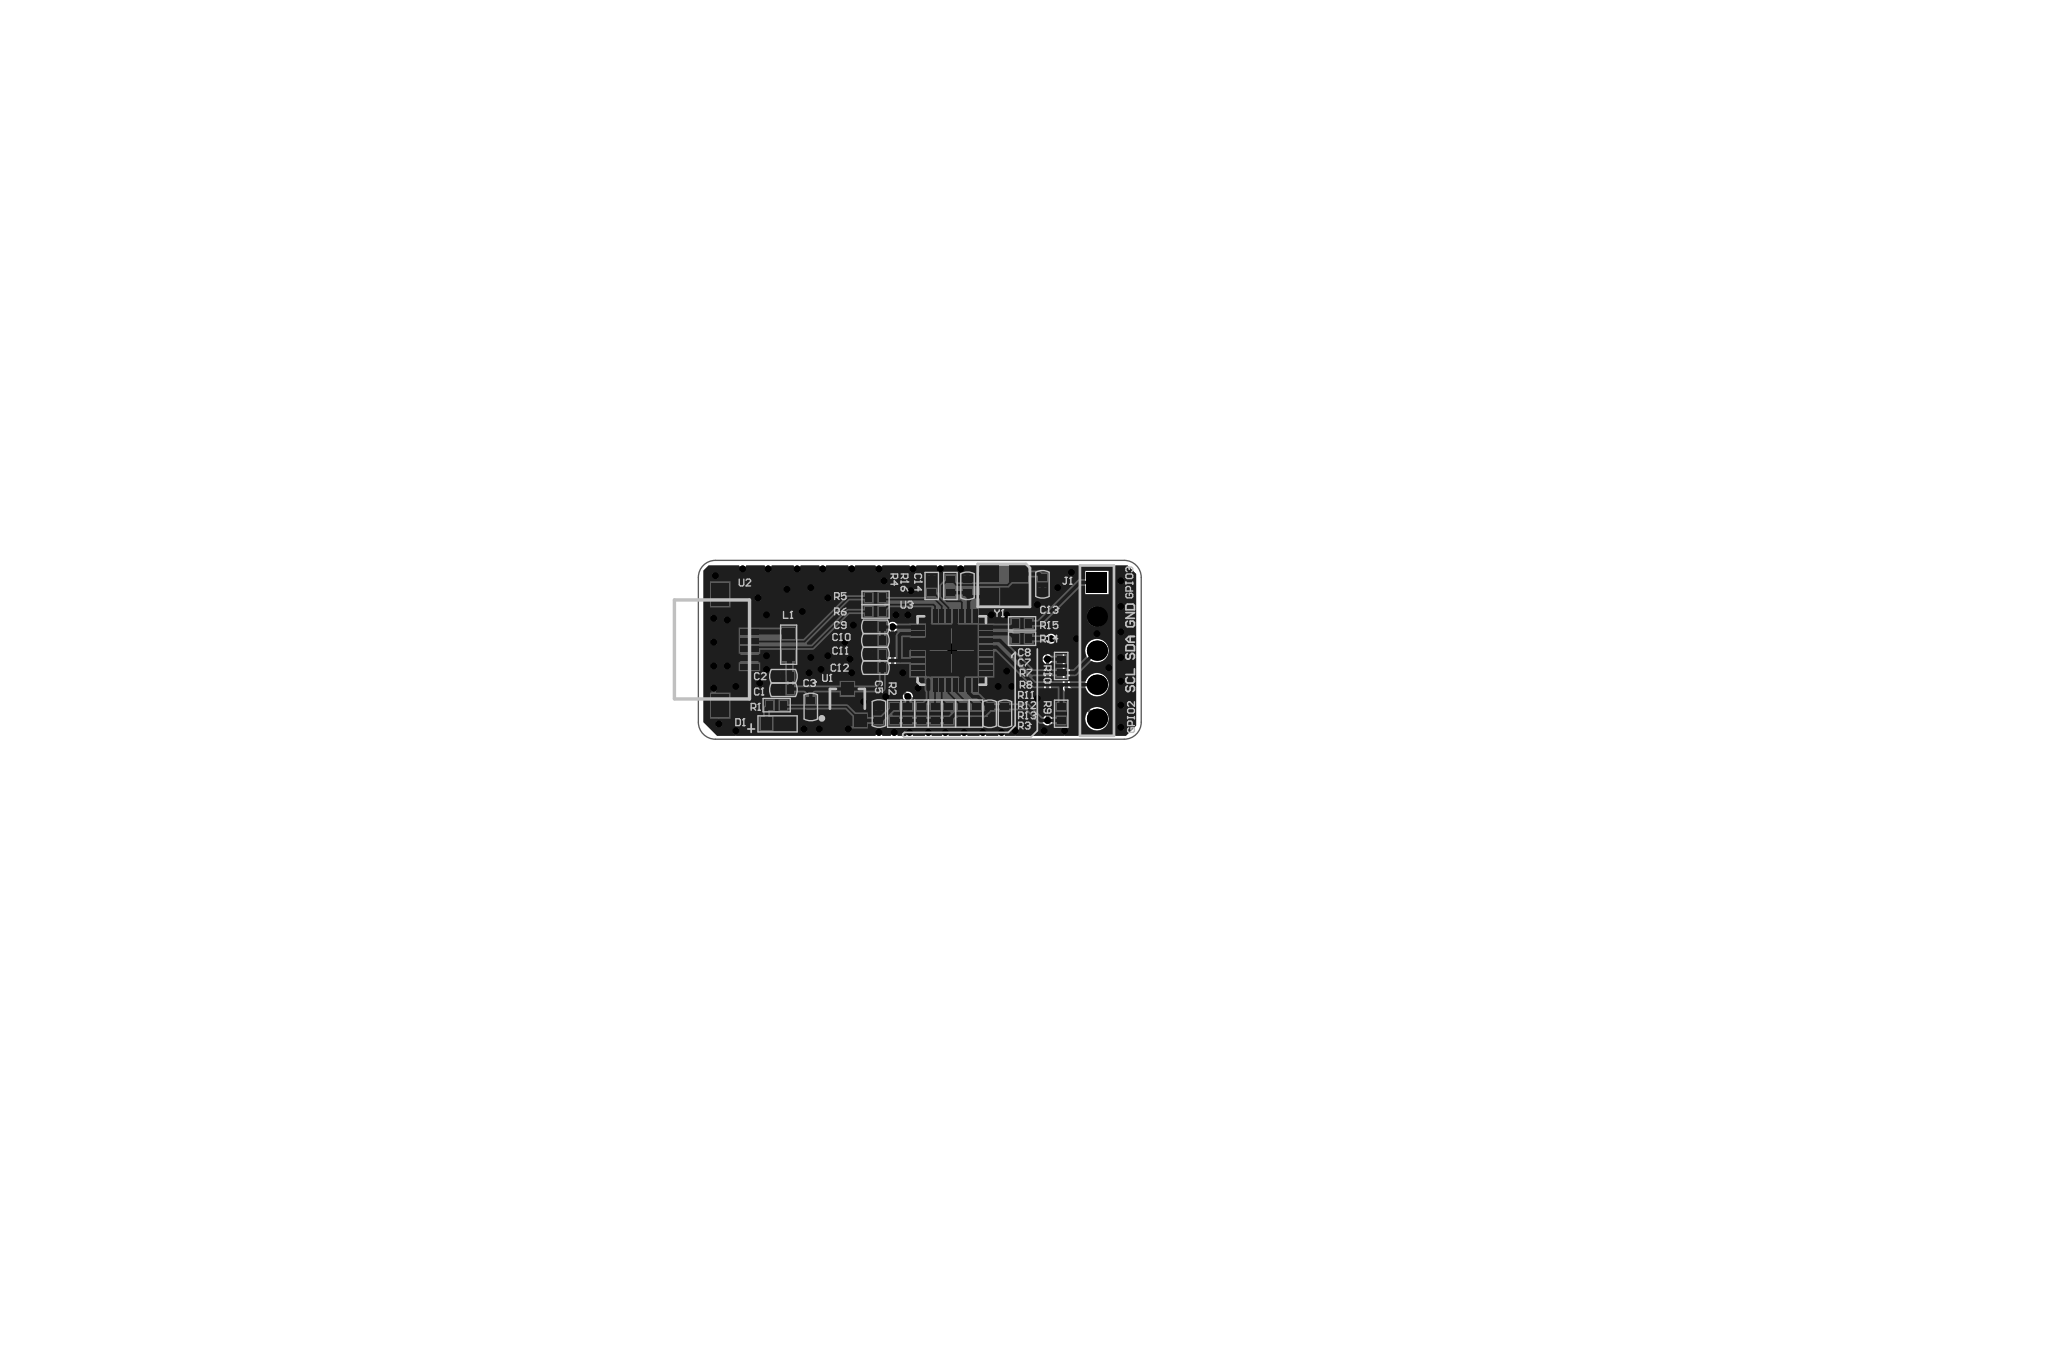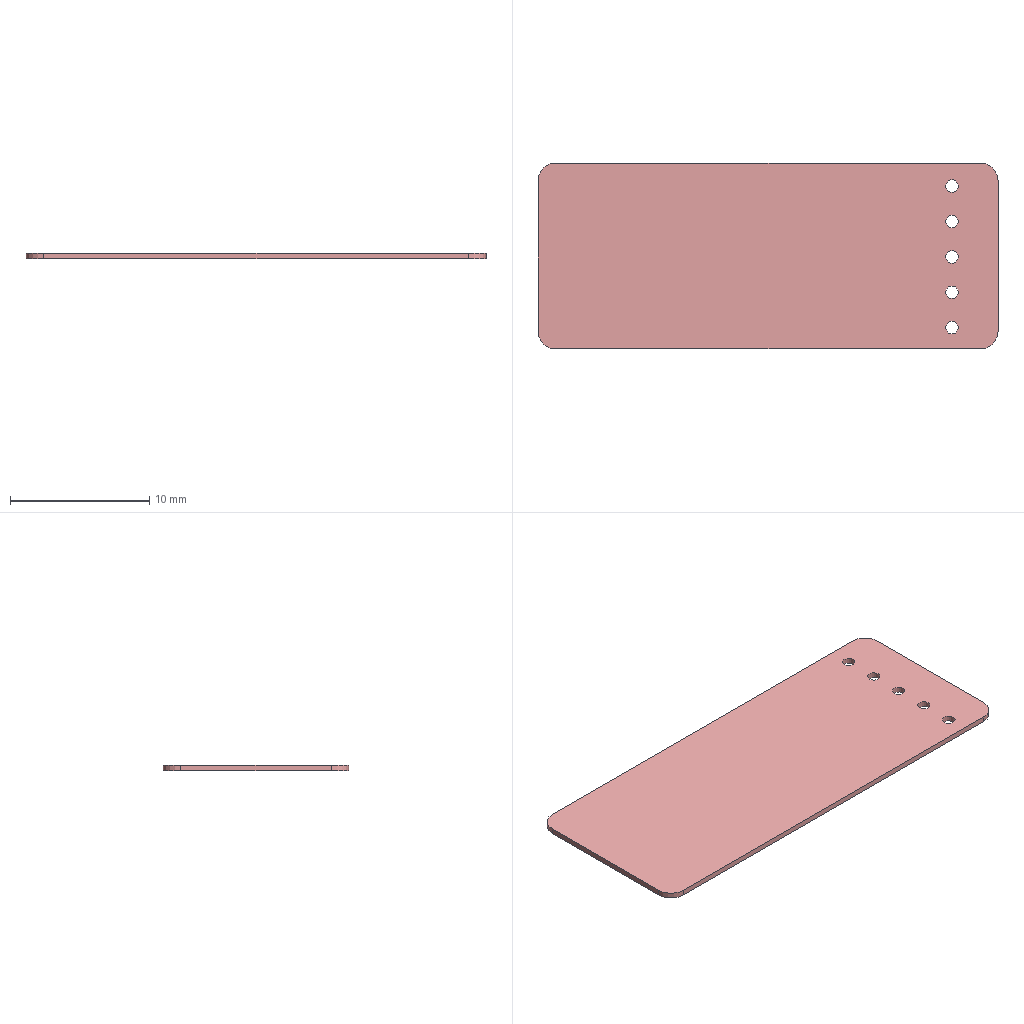Circuit board layout | Altium Designer | box 33 x 13.3 x 0.4 mm
Layer stack:
# Altium Designer layer stack of  (unit mm; dielectric type: 0 none, 1 core, 2 prepreg, 3 surface material)
index,name,kind,layer,copper_thickness_mm,dielectric_type,dielectric_thickness_mm,dielectric_material,dielectric_constant
0,Top Paste,other,,,,,,
1,Top Overlay,other,,,,,,
2,Top Solder,dielectric,,,3,0.0102,Solder Resist,3.5
3,Top Layer,copper,Top Layer,0.0356,,,,
4,Dielectric 1,dielectric,,,0,0.32,FR-4,4.8
5,Bottom Layer,copper,Bottom Layer,0.0356,,,,
6,Bottom Solder,dielectric,,,3,0.0102,Solder Resist,3.5
7,Bottom Overlay,other,,,,,,
8,Bottom Paste,other,,,,,,
# drill layer pairs: low layer,high layer
drill_pair,Top Layer,Bottom Layer
Part placement:
Designator,Comment,Layer,Footprint,Center-X(mm),Center-Y(mm),Rotation
Y1,12M,TopLayer,XTAL_3225,22.776,11.469,180
U3,FT4222,TopLayer,QFN32,18.895,6.614,90
U2,USB,TopLayer,MicroUSB,2.721,6.651,270
U1,AX6601,TopLayer,SOT_23,11.11,2.572,0
R16,1M,TopLayer,R0402,18.796,11.43,270
R15,000R,TopLayer,R0402,24.13,8.636,0
R14,000R,TopLayer,R0402,24.13,7.493,0
R13,10K,TopLayer,R0402,16.637,1.905,90
R12,10K,TopLayer,R0402,17.653,1.905,90
R11,10K,TopLayer,R0402,18.669,1.905,90
R10,1K,TopLayer,R0402,27.051,5.461,90
R9,1K,TopLayer,R0402,27.051,1.905,270
R8,000R,TopLayer,R0402,19.685,1.905,90
R7,000R,TopLayer,R0402,20.701,1.905,90
R6,000R,TopLayer,R0402,13.208,9.525,0
R5,000R,TopLayer,R0402,13.208,10.541,0
R4,12K,TopLayer,R0402,17.399,11.43,270
R3,NC,TopLayer,R0402,15.621,1.905,270
R2,000R,TopLayer,R0402,14.605,1.905,270
R1,470ohm,TopLayer,R0402,5.842,2.54,180
L1,000R,TopLayer,R0603,6.731,7.048,90
J1,PIN 2.54*5,TopLayer,DIP2.54*5,29.718,6.604,270
D1,Led,TopLayer,R0603,5.905,1.143,180
C14,20pF,TopLayer,C0402,20.066,11.43,270
C13,20pF,TopLayer,C0402,25.654,11.557,90
C12,0.1uF,TopLayer,C0402,13.208,5.334,0
C11,4.7uF,TopLayer,C0402,13.208,6.35,0
C10,0.1uF,TopLayer,C0402,13.208,7.366,0
C9,4.7uF,TopLayer,C0402,13.208,8.382,0
C8,0.1uF,TopLayer,C0402,22.86,1.905,90
C7,4.7uF,TopLayer,C0402,21.717,1.905,90
C5,4.7uF,TopLayer,C0402,13.462,1.905,270
C3,4.7uF,TopLayer,C0402,8.382,2.413,90
C2,0.1uF,TopLayer,C0402,6.35,4.699,0
C1,4.7uF,TopLayer,C0402,6.35,3.683,0
Pad and via stacks:
# Altium Designer via and pad stacks of  (unit mm). Each distinct definition once, with the count of objects using it.
# via: kind,start_layer,end_layer,hole_mm,diameter_mm,mode(0 simple;1 top-mid-bottom;2 full stack),diameter_per_layer,count,example_net
# pad: kind,layer,hole_mm,hole_type(0 round;1 square;2 slot),plating,top_size,top_shape(1 round;2 rect;3 octagon;9 rounded rect),mid_size,bottom_size,mode,footprint,size_per_layer,count,example
pad,Top Layer,0,0,plated,1.6x1.6,2,1.6x1.6,1.6x1.6,0,QFN32,,4,U3.33
pad,Top Layer,0,0,plated,0.3x1,2,0.3x1,0.3x1,0,QFN32,,31,U3.20
pad,Top Layer,0,0,plated,0.3x1,1,0.3x1,0.3x1,0,QFN32,,1,U3.1
pad,Top Layer,0,0,plated,0.6x0.5,2,0.6x0.5,0.6x0.5,0,R0402,,32,R13.2
pad,Top Layer,0,0,plated,0.6x0.5,2,0.6x0.5,0.6x0.5,0,C0402,,24,C12.1
pad,Top Layer,0,0,unplated,0.9x0.8,2,0.9x0.8,0.9x0.8,0,R0603,,4,L1.1
pad,Top Layer,0,0,plated,0.9x0.95,2,0.9x0.95,0.9x0.95,0,SOT_23,,3,U1.1
pad,Top Layer,0,0,plated,1.4x1.2,2,1.4x1.2,1.4x1.2,0,XTAL_3225,,4,Y1.1
pad,Top Layer,0,0,plated,1.28x1.7,2,1.28x1.7,1.28x1.7,0,MicroUSB,,2,U2.0
pad,Top Layer,0,0,plated,1.35x0.4,2,1.35x0.4,1.35x0.4,0,MicroUSB,,5,U2.5
pad,Multi-Layer,0.9,0,plated,1.5x1.5,1,1.5x1.5,1.5x1.5,0,DIP2.54*5,,3,J1.4
pad,Multi-Layer,0.9,0,plated,1.5x1.5,2,1.5x1.5,1.5x1.5,0,DIP2.54*5,,1,J1.1
pad,Multi-Layer,0.8992,0,plated,1.499x1.499,1,1.499x1.499,1.499x1.499,0,DIP2.54*5,,1,J1.5
via,Top Layer,Bottom Layer,0.254,0.508,0,,82,VCC3V3
via,Top Layer,Bottom Layer,0.381,0.762,0,,5,GND
Copper pours:
name,layer,net,type(0 solid;1 hatched;2 none)
GND Layer-No Net,Bottom Layer,GND,0
GND Layer-No Net,Top Layer,GND,0
Design rules, without the lines most boards share:
# Altium Designer design rules of  (exported by Altium Designer, unit mm)
# columns: name | kind | enabled | priority | scope1 | scope2 | descriptor | typed fields (field=value)
SilkToSilkClearance | 55 | disabled | 1 | All | All | Silk to Silk (Clearance=0mil) (Disabled)(All),(All) |
ComponentClearance | 24 | disabled | 1 | All | All | Component Clearance Constraint ( Horizontal Gap = 0mil, Vertical Gap = 0mil ) (Disabled)(All),(All)  | gap=0
NetAntennae | 56 | disabled | 1 | All | All | Net Antennae (Tolerance=0mil) (Disabled)(All) |
SilkToBoardRegionClearance | 59 | disabled | 1 | All | All | Silk primitive without silk layer |
SilkToSolderMaskClearance | 54 | disabled | 1 | IsPad | All | Silk To Solder Mask (Clearance=0mil) (Disabled)(IsPad),(All) |
SolderMaskExpansion | 13 | disabled | 1 | All | All | Solder Mask Expansion (Expansion =4mil) (Disabled)(All) | expansion=0.1016
PasteMaskExpansion | 14 | disabled | 1 | All | All | Paste Mask Expansion (Expansion =0mil) (Disabled)(All) | expansion=0
Clearance | 0 | enabled | 1 | All | All | Clearance Constraint (Gap=5mil) (All),(All) | gap=0.127
PlaneConnect | 6 | disabled | 1 | All | All | Power Plane Connect Rule(Direct Connect )(Expansion=20mil) (Conductor Width=10mil) (Air Gap=10mil) (Entries=4) (Disabled)(All) | relief_conductor_width=0.254 relief_entries=4 relief_expansion=0.508
PlaneClearance | 12 | disabled | 1 | All | All | Power Plane Clearance (Clearance =5mil) (Disabled)(All) | clearance=0.127
PolygonConnect | 20 | disabled | 1 | All | All | Polygon Connect Rule(Direct Connect )(Conductor Width=10mil) (Relief Angle=90 Angle) (Entries=4) (Air Gap Width=10mil) (Disabled)(All),(All) | connect_style(0=relief,1=direct,2=none)=1 relief_conductor_width=0.254 relief_entries=4
Width | 2 | enabled | 1 | All | All | Width Constraint (Min=5mil) (Max=50mil) (Preferred=10mil) (All) |
RoutingPriority | 8 | disabled | 1 | All | All | TRoutingPriorityRule(Priority=0) (Disabled)(All) |
RoutingLayers | 9 | disabled | 1 | All | All | Routing Layers(Disabled)(All) |
RoutingCorners | 10 | disabled | 1 | All | All | Routing Corners (Style=45-Degree) (Min Setback=100mil) (Max Setback=100mil) (Disabled)(All) |
RoutingVias | 11 | enabled | 1 | All | All | Routing Via (MinHoleWidth=5mil) (MaxHoleWidth=30mil) (PreferredHoleWidth=10mil) (MinWidth=5mil) (MaxWidth=50mil) (PreferedWidth=20mil) (All) | via_min_hole=0.127 via_max_hole=0.762 via_preferred_diameter=0.508 via_preferred_hole=0.254
RoutingTopology | 7 | disabled | 1 | All | All | Routing Topology Rule(Topology=Shortest) (Disabled)(All) |
FabricationTestPointUsage | 44 | disabled | 1 | All | All | Fabrication Testpoint Usage (Valid =One Required, Allow multiple per net=No) (Disabled)(All) |
FabricationTestpoint | 43 | disabled | 1 | All | All | Fabrication Testpoint Style (Under Component=Yes) (Disabled)(All) |
AssemblyTestPointUsage | 58 | disabled | 1 | All | All | Assembly Testpoint Usage (Valid =One Required, Allow multiple per net=No) (Disabled)(All) |
AssemblyTestpoint | 57 | disabled | 1 | All | All | Assembly Testpoint Style (Under Component=Yes) (Disabled)(All) |
Height | 50 | disabled | 1 | All | All | Height Constraint (Min=0mil) (Max=1000mil) (Prefered=500mil) (Disabled)(All) | min_height=0 max_height=25.4
LayerPairs | 48 | disabled | 1 | All | All | Pads and Vias to follow the Drill pairs settings |
HoleSize | 42 | disabled | 1 | All | All | Hole Size Constraint (Min=1mil) (Max=100mil) (Disabled)(All) |
Fanout_Default | 49 | disabled | 5 | All | All | Fanout Control Rule ( (Disabled)(All) ) |
Fanout_Small | 49 | disabled | 4 | (CompPinCount < 5) | All | Fanout Control Rule ( (Disabled)((CompPinCount < 5)) ) |
Fanout_SOIC | 49 | disabled | 3 | IsSOIC | All | Fanout Control Rule ( (Disabled)(IsSOIC) ) |
Fanout_LCC | 49 | disabled | 2 | IsLCC | All | Fanout Control Rule ( (Disabled)(IsLCC) ) |
Fanout_BGA | 49 | disabled | 1 | IsBGA | All | Fanout Control Rule ( (Disabled)(IsBGA) ) |
DiffPairsRouting | 51 | disabled | 1 | All | All | Differential Pairs Uncoupled Length using the Gap Constraints (Min=10mil) (Max=10mil) (Prefered=10mil)  and Width Constraints (Min=15mil) (Max=15mil) (Prefered=15mil) (Disabled)(All) |
HoleToHoleClearance | 52 | disabled | 1 | All | All | Hole To Hole Clearance (Gap=10mil) (Disabled)(All),(All) | gap=0.254
MinimumSolderMaskSliver | 53 | disabled | 1 | All | All | Minimum Solder Mask Sliver (Gap=10mil) (Disabled)(All),(All) |
Classes set for this board:
# Altium Designer classes of  (member kind: 0 net, 1 component, 2 from-to, 3 pad, 4 layer, 5 differential pair, 6 design channel, 7 polygon, 8 structure, 9 xSignal)
# columns: class name | member kind | superclass | members
FT4222_Dongle_V1.0 | 1 | no | C1; C2; C3; C5; C7; C8; C9; C10; C11; C12; C13; C14; D1; J1; L1; R1; R2; R3; R4; R5; R6; R7; R8; R9; R10; R11; R12; R13; R14; R15; R16; U1; U2; U3; Y1;